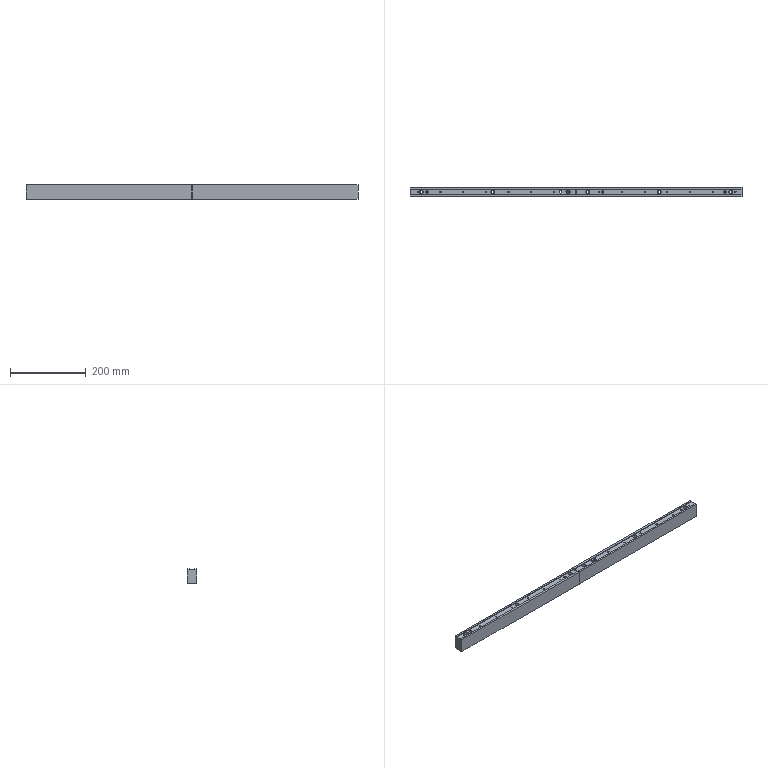Part | 2 solids | 76 faces | box 878 x 25 x 39 mm | volume 812012 mm3 | cylinder 32 | plane 30 | cone 14 | commonest cylinder face diameters 3.3 x14 6 x6 6.6 x6 11 x6